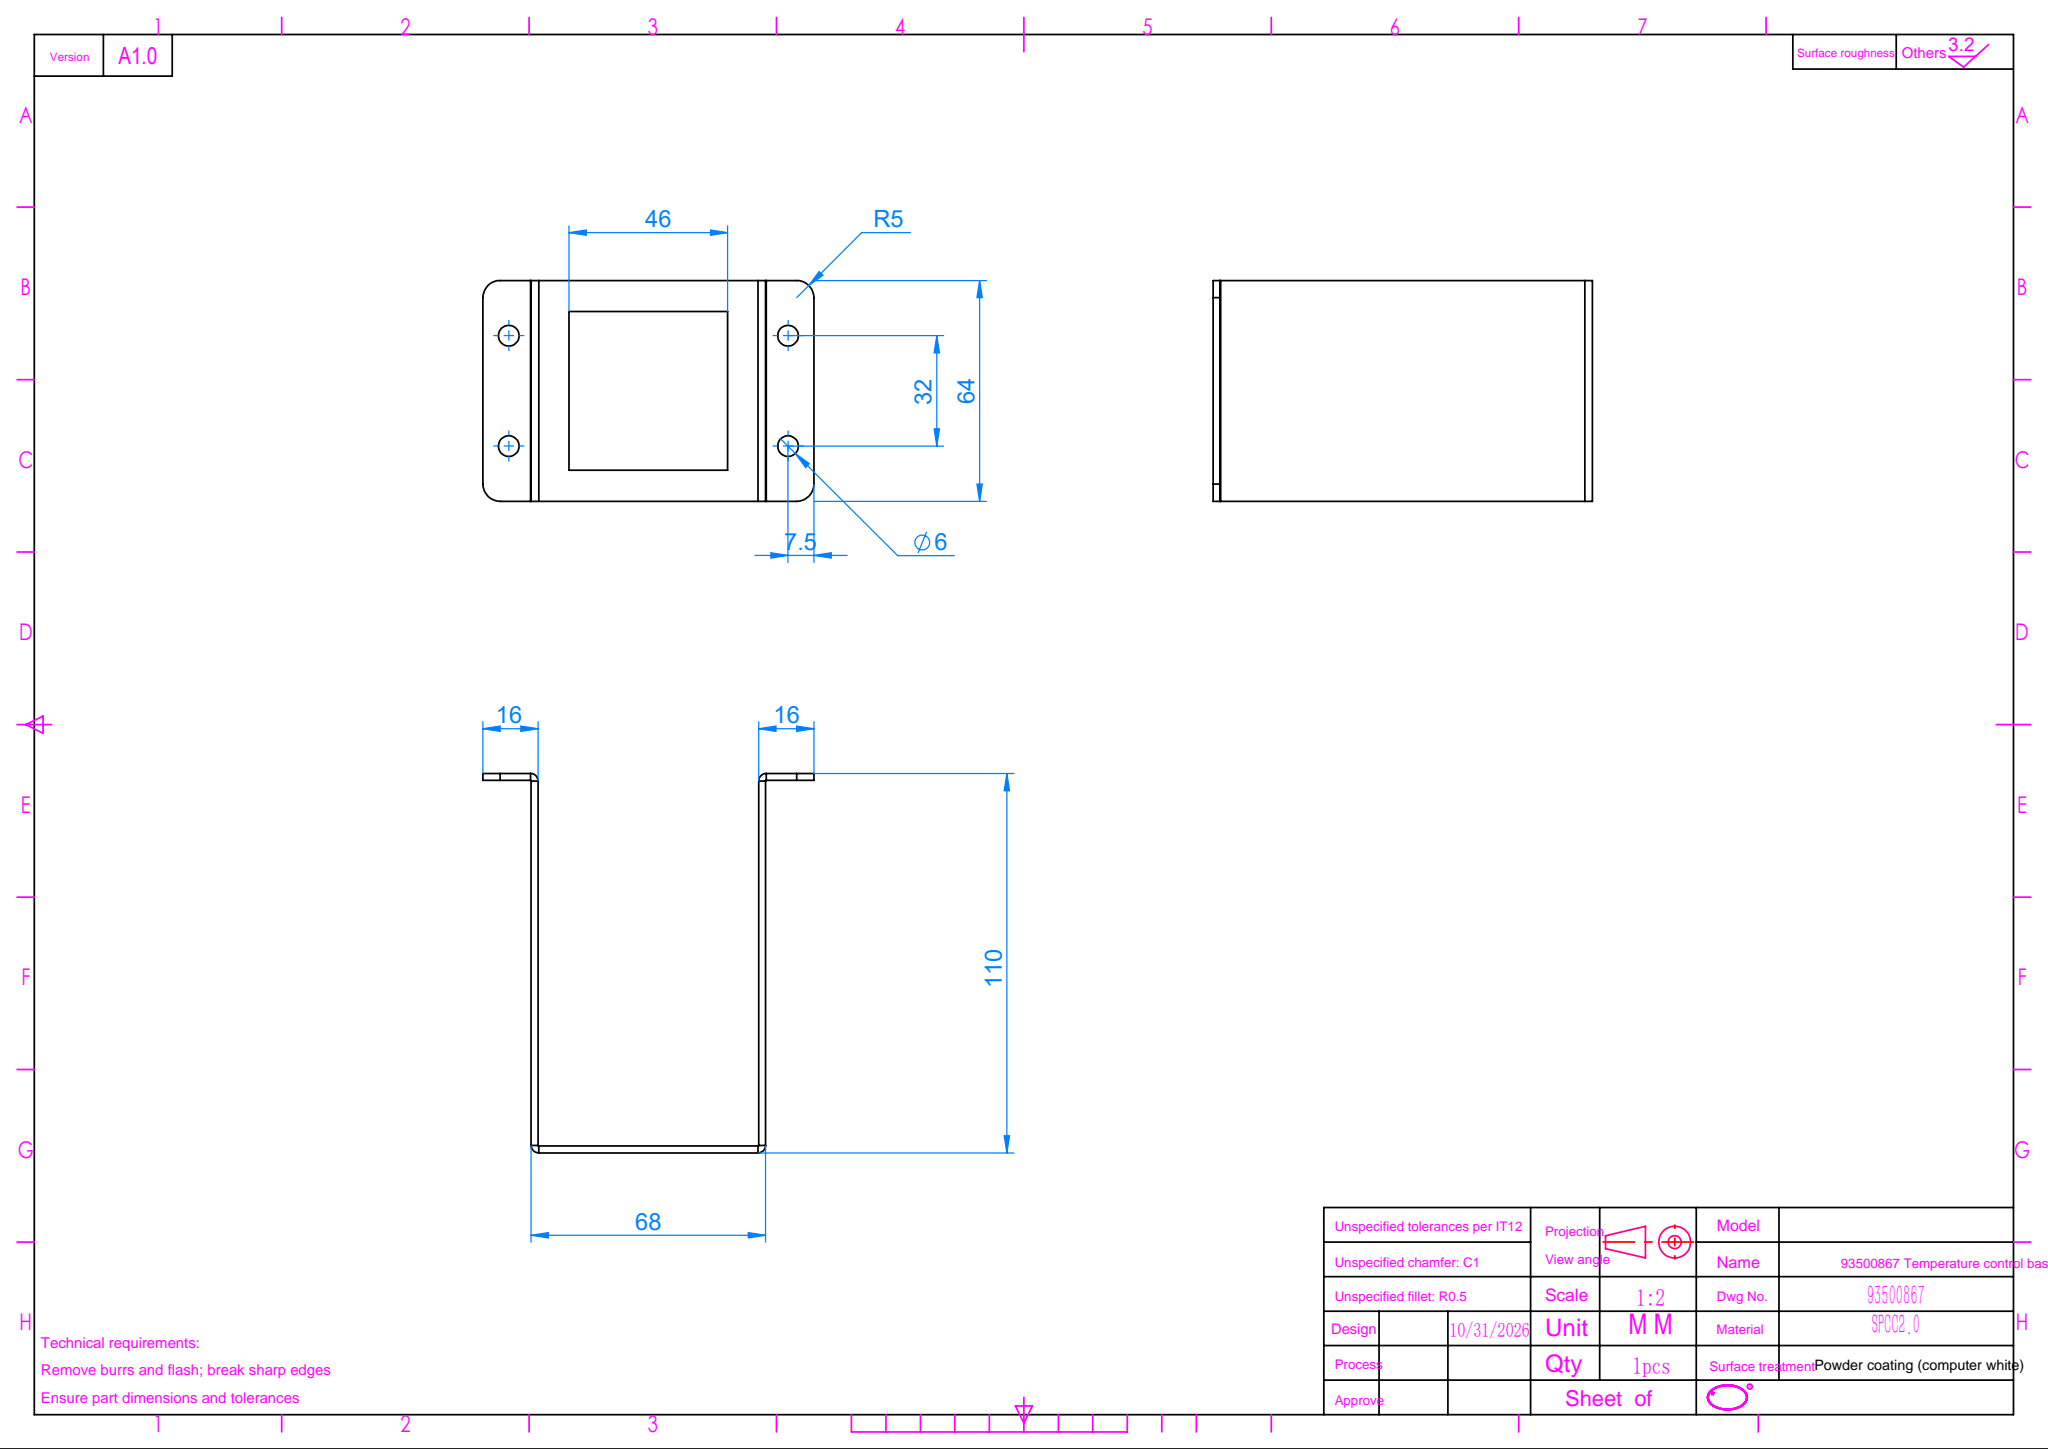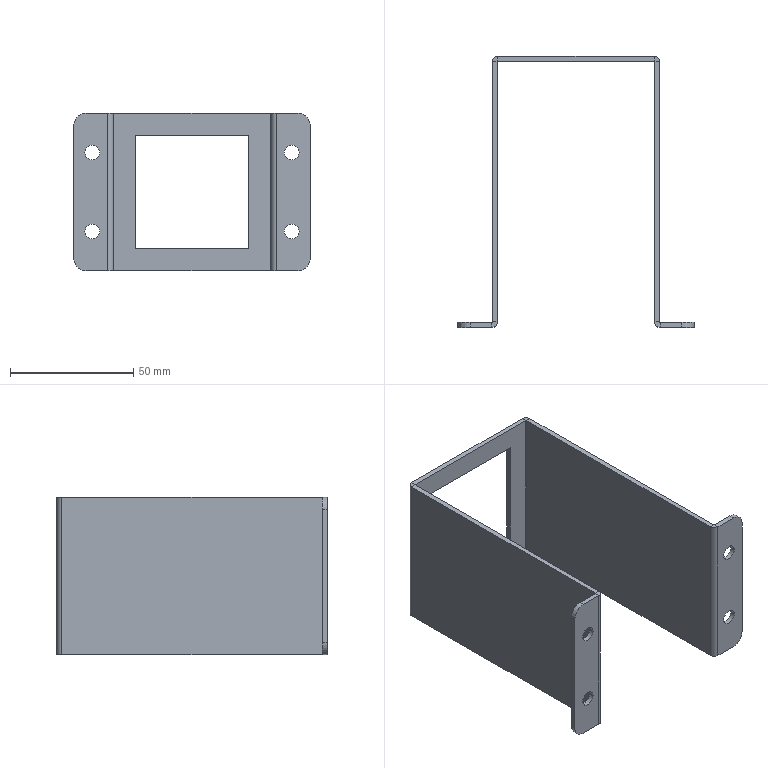Part | SolidWorks | features ICE 2, Fillet 1, FlatPattern 1, SMBaseFlange 1, SheetMetal 1 | 1 solid | 54 faces | box 96 x 110 x 64 mm | volume 35171 mm3 | plane 34 | cylinder 20 | commonest cylinder face diameters 6 x8 0.4 x4 4.4 x4 10 x4